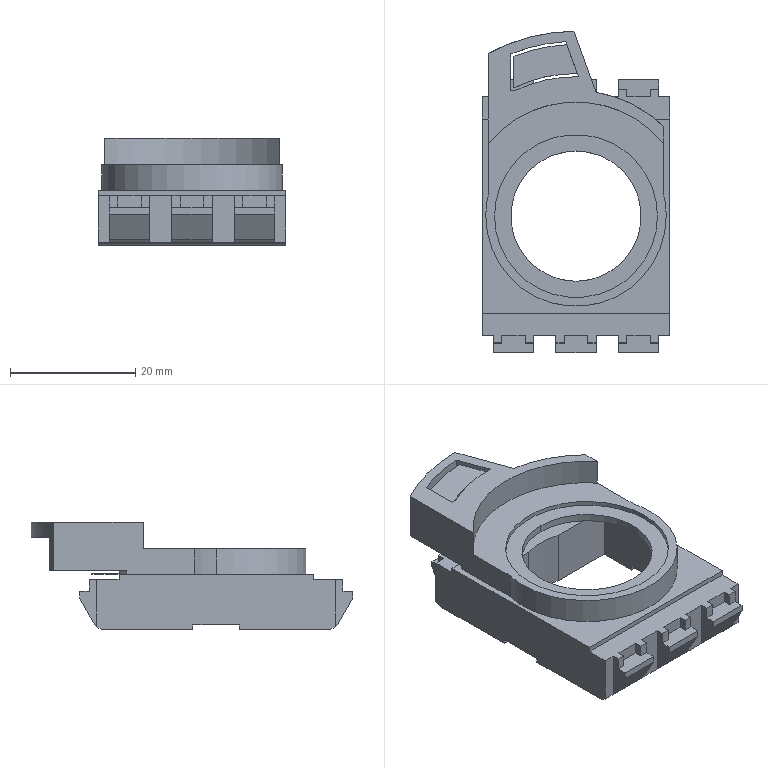Part | STEP file | A22NZ_H_01 | 1 solid | 172 faces | box 30 x 51.298 x 17.1 mm | volume 5961 mm3 | plane 151 | cylinder 21 | commonest cylinder face diameters 20.8 x5 28.8 x3 4 x2 25.4 x2 26 x2 36.4 x1